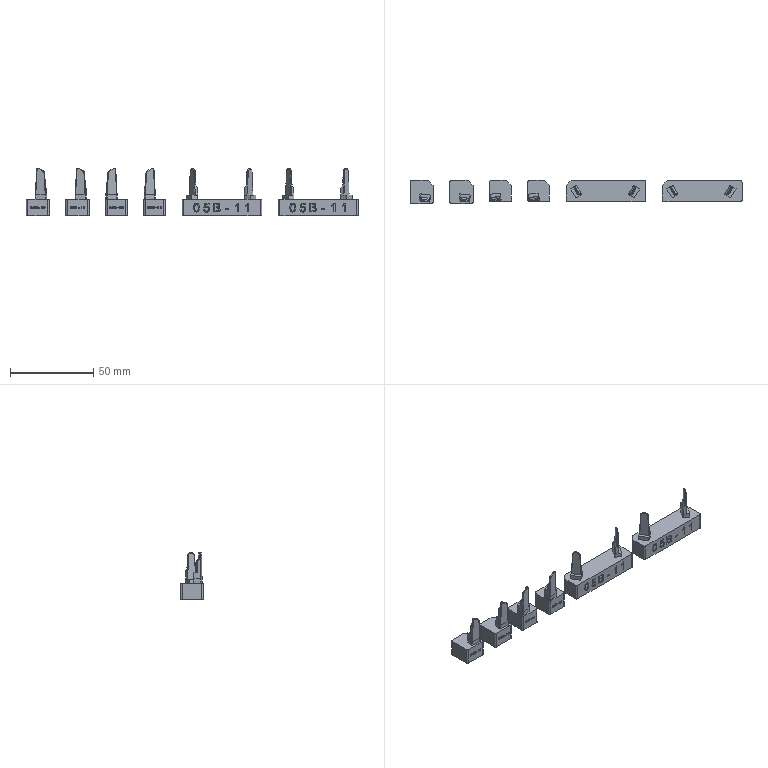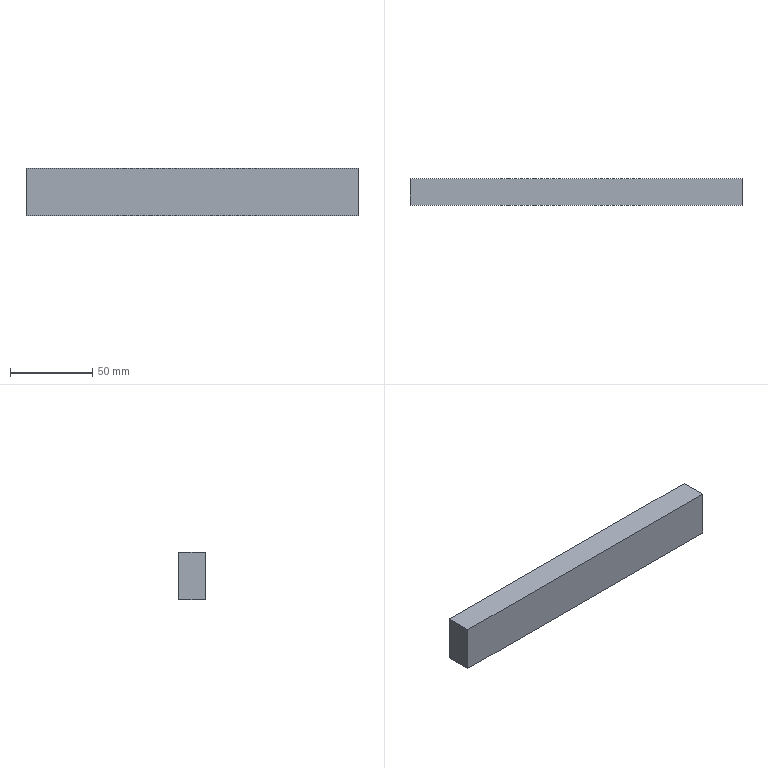CAM job | NX | 3-axis milling | part box 200 x 14 x 28.763 mm | stock box 202 x 16 x 28.966 mm
Tools:
number,name,description,diameter,corner_radius,flute_length,length,flutes
0,D8-0.075,Milling Tool-5 Parameters,7.85,0.0,50.0,75.0,2
0,D4R2,Milling Tool-Ball Mill,4.0,2.0,50.0,75.0,2
Operations:
program,operation,operation_type,tool,method,geometry_group,spindle_rpm,surface_speed,feed_per_tooth,feed_cut,feed_plunge,cut_length_mm,path_length_mm,cut_time_min,machine_time_min
05B-10F1,CAVITY_MILL_C_0_0,CavityMilling,D8-0.075,MILL_ROUGH,05B-10_WP,10000.0,0.0,0.0,4500.0,0.0,104709.031,105770.631,23.144,23.25
05B-10F1,CAVITY_PLANAR_MILL_1_0,PlanarMilling,D8-0.075,METHOD,05B-10_WP,10000.0,0.0,0.0,4500.0,0.0,3179.434,3323.177,0.7065,0.7209
05B-10F1,CAVITY_PLANAR_MILL_1_1,PlanarMilling,D8-0.075,METHOD,05B-10_WP,10000.0,0.0,0.0,4500.0,0.0,5423.422,5567.177,1.205,1.22
05B-10F1,CAVITY_PLANAR_MILL_1_2,PlanarMilling,D8-0.075,METHOD,05B-10_WP,10000.0,0.0,0.0,4500.0,0.0,3043.438,3187.177,0.6763,0.6907
05B-10F1,CAVITY_PLANAR_MILL_1_3,PlanarMilling,D8-0.075,METHOD,05B-10_WP,10000.0,0.0,0.0,4500.0,0.0,5423.428,5567.177,1.205,1.22
05B-10F1,CAVITY_PLANAR_MILL_1_4,PlanarMilling,D8-0.075,METHOD,05B-10_WP,10000.0,0.0,0.0,4500.0,0.0,3043.438,3187.177,0.6763,0.6907
05B-10F1,CAVITY_PLANAR_MILL_1_5,PlanarMilling,D8-0.075,METHOD,05B-10_WP,10000.0,0.0,0.0,4500.0,0.0,3179.434,3323.177,0.7065,0.7209
05B-10F2,FACE_MILLING_BASE_0_0,FaceMilling,D8-0.075,METHOD,05B-10_WP,10000.0,0.0,0.0,1000.0,0.0,1540.876,1587.609,1.54,1.544
05B-10F2,PLANAR_MILL_BASE_0_0,PlanarMilling,D8-0.075,MILL_FINISH,05B-10_WP,10000.0,0.0,0.0,1000.0,0.0,250.103,367.636,0.2501,0.2619
05B-10F2,PLANAR_MILL_BASE_0_1,PlanarMilling,D8-0.075,MILL_FINISH,05B-10_WP,10000.0,0.0,0.0,1000.0,0.0,448.103,565.636,0.4481,0.4599
05B-10F2,PLANAR_MILL_BASE_0_2,PlanarMilling,D8-0.075,MILL_FINISH,05B-10_WP,10000.0,0.0,0.0,1000.0,0.0,238.103,355.636,0.2381,0.2499
05B-10F2,PLANAR_MILL_BASE_0_3,PlanarMilling,D8-0.075,MILL_FINISH,05B-10_WP,10000.0,0.0,0.0,1000.0,0.0,448.103,565.636,0.4481,0.4599
05B-10F2,PLANAR_MILL_BASE_0_4,PlanarMilling,D8-0.075,MILL_FINISH,05B-10_WP,10000.0,0.0,0.0,1000.0,0.0,238.103,355.636,0.2381,0.2499
05B-10F2,PLANAR_MILL_BASE_0_5,PlanarMilling,D8-0.075,MILL_FINISH,05B-10_WP,10000.0,0.0,0.0,1000.0,0.0,250.103,367.636,0.2501,0.2619
05B-10F3,CONTOUR_AREA_0_0,SurfaceContour,D4R2,MILL_FINISH,05B-10_WP,13000.0,163.0,0.0769,2000.0,100.0,10088.925,10365.04,5.045,5.072
05B-10F4,ZLEVEL_PROFILE_CLIMB_0_0,ZLevelMilling,D8-0.075,MILL_FINISH,05B-10_WP,10000.0,0.0,0.0,4000.0,0.0,43838.687,44907.791,10.96,11.067
05B-10F4,PLANAR_MILL_BASE_0_0_COPY,PlanarMilling,D8-0.075,MILL_FINISH,05B-10_WP,10000.0,0.0,0.0,1000.0,0.0,486.146,1454.616,0.4861,0.583
05B-10F4,PLANAR_MILL_BASE_0_0_COPY_1,PlanarMilling,D8-0.075,MILL_FINISH,05B-10_WP,10000.0,0.0,0.0,1000.0,0.0,92.885,210.418,0.0929,0.1046
05B-10F4,PLANAR_MILL_BASE_0_1_COPY,PlanarMilling,D8-0.075,MILL_FINISH,05B-10_WP,10000.0,0.0,0.0,1000.0,0.0,158.885,276.418,0.1589,0.1706
05B-10F4,PLANAR_MILL_BASE_0_2_COPY,PlanarMilling,D8-0.075,MILL_FINISH,05B-10_WP,10000.0,0.0,0.0,1000.0,0.0,88.885,206.418,0.0889,0.1006
05B-10F4,PLANAR_MILL_BASE_0_3_COPY,PlanarMilling,D8-0.075,MILL_FINISH,05B-10_WP,10000.0,0.0,0.0,1000.0,0.0,158.885,276.418,0.1589,0.1706
05B-10F4,PLANAR_MILL_BASE_0_4_COPY,PlanarMilling,D8-0.075,MILL_FINISH,05B-10_WP,10000.0,0.0,0.0,1000.0,0.0,88.885,206.418,0.0889,0.1006
05B-10F4,PLANAR_MILL_BASE_0_5_COPY,PlanarMilling,D8-0.075,MILL_FINISH,05B-10_WP,10000.0,0.0,0.0,1000.0,0.0,92.885,210.418,0.0929,0.1046